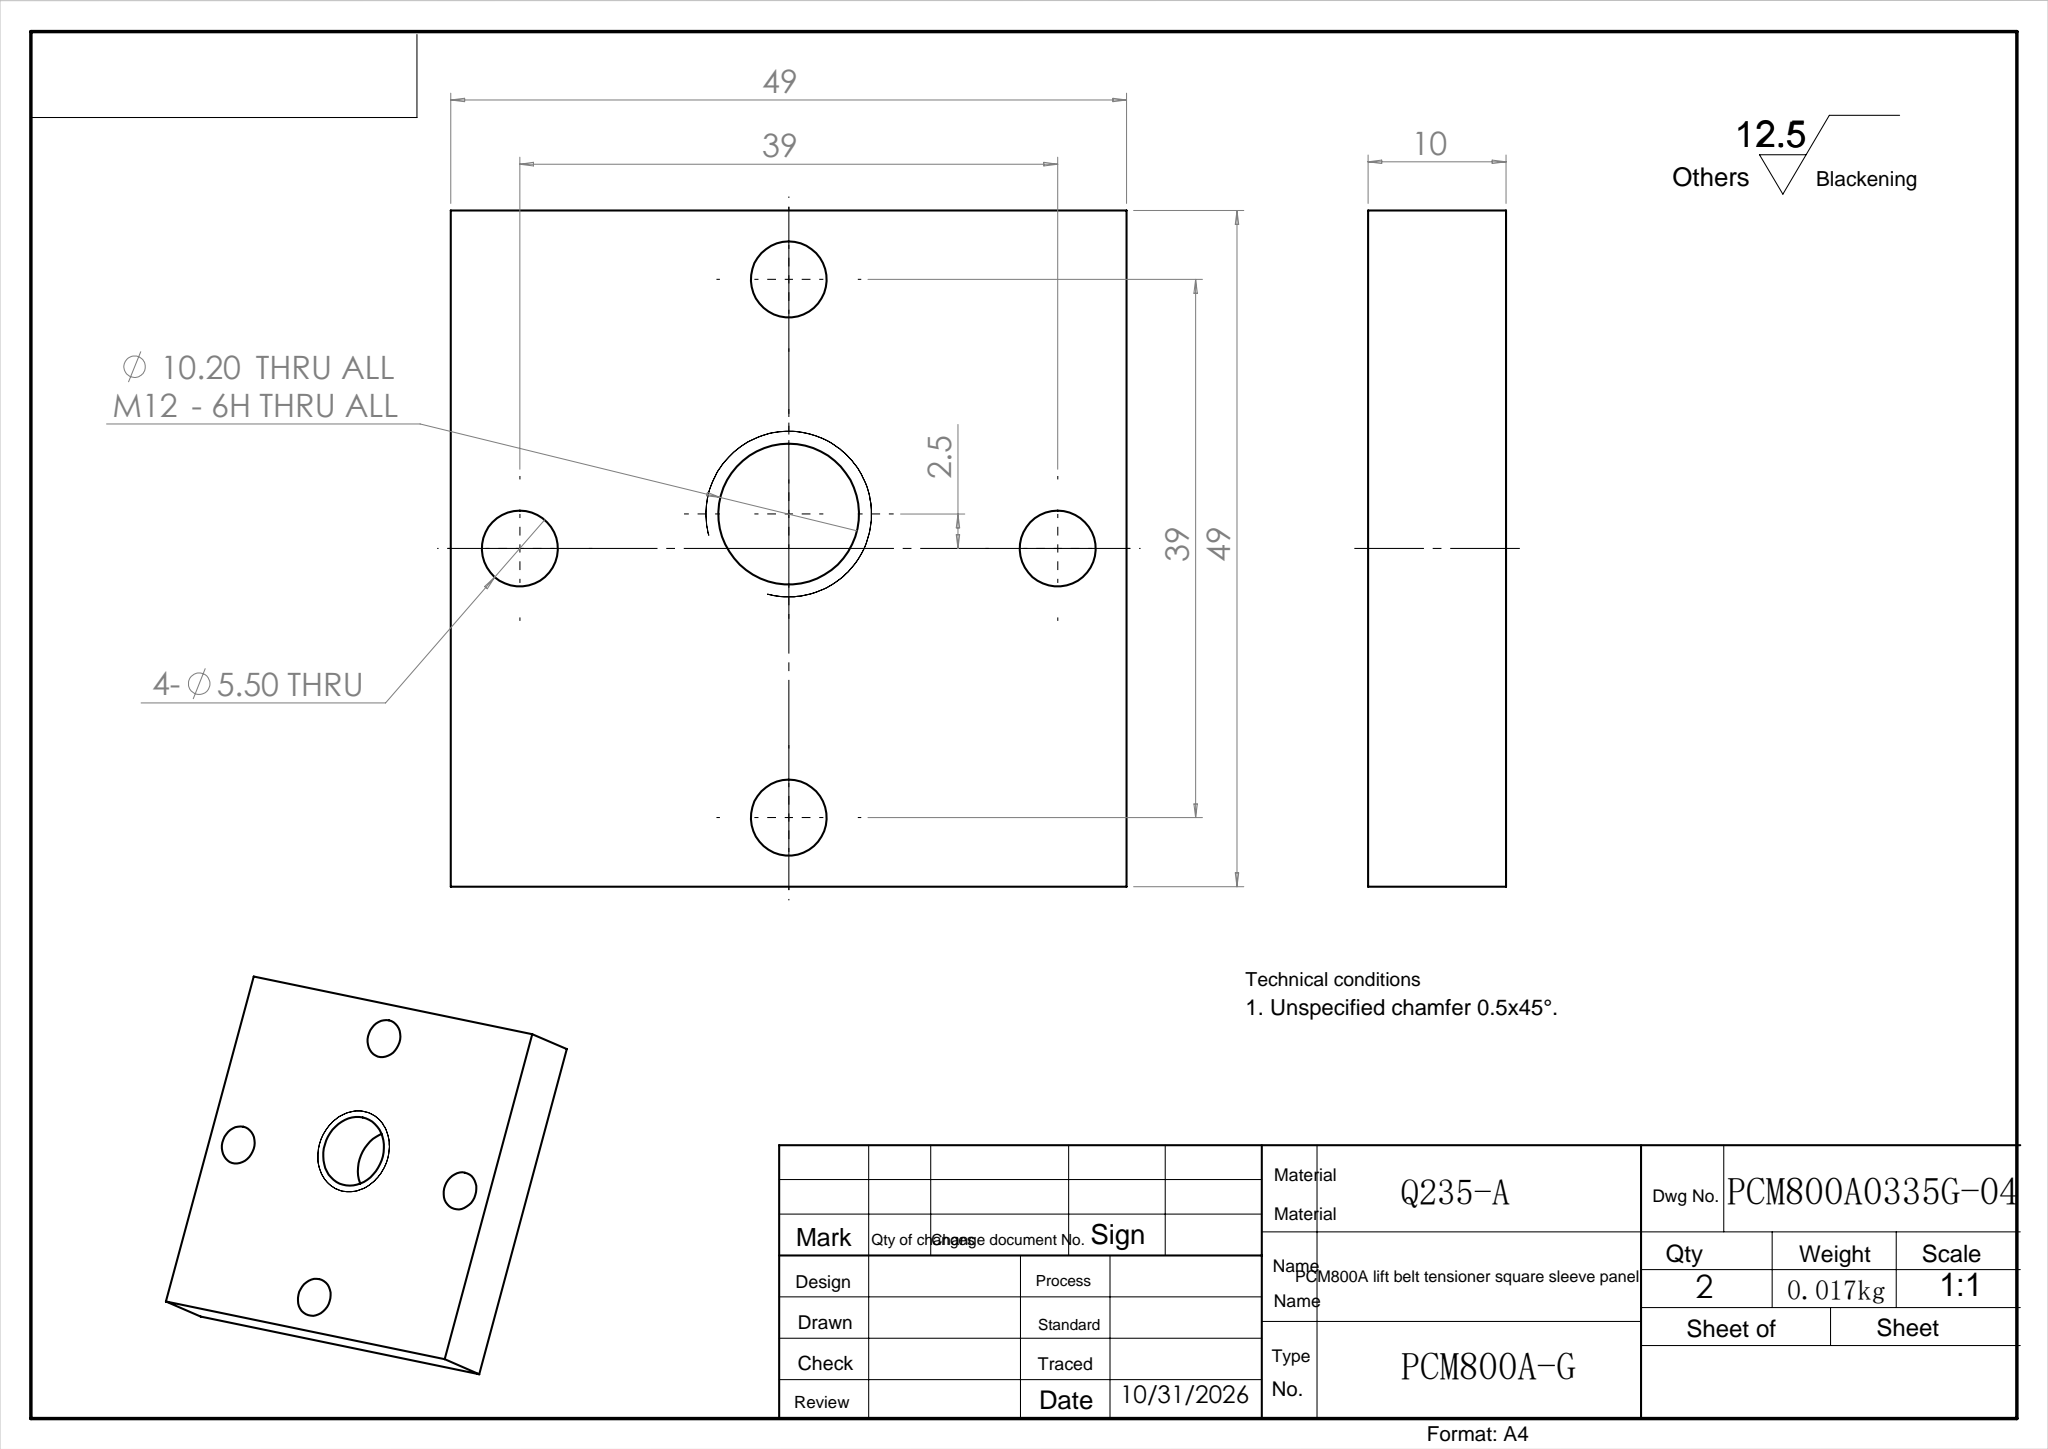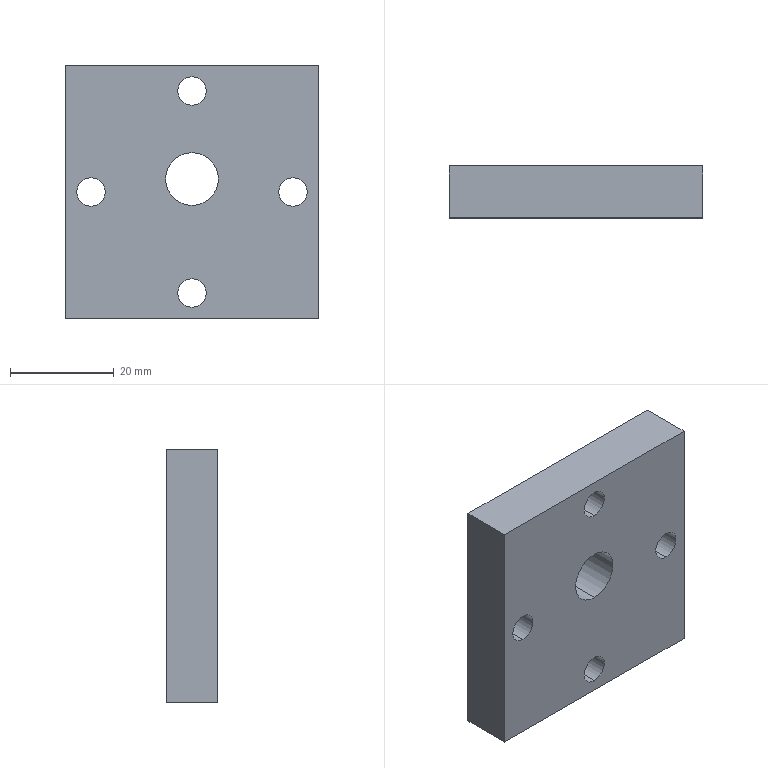Part | SolidWorks | features 3DProfileFeature 1, Cut 1, Extrusion 1, HoleWzd 1 | 1 solid | 16 faces | box 49 x 10 x 49 mm | volume 22243 mm3 | cylinder 10 | plane 6 | commonest cylinder face diameters 5.5 x8 10.2 x2
STEP:
#1=CARTESIAN_POINT('',(24.5,0.,-27.1));
#2=VERTEX_POINT('',#1);
#3=CARTESIAN_POINT('',(24.5,0.,-16.9));
#4=VERTEX_POINT('',#3);
#5=CARTESIAN_POINT('',(24.5,0.,-22.));
#6=DIRECTION('',(0.,1.,0.));
#7=DIRECTION('',(0.,0.,1.));
#8=AXIS2_PLACEMENT_3D('',#5,#6,#7);
#9=CIRCLE('',#8,5.1);
#10=EDGE_CURVE('',#2,#4,#9,.T.);
#11=ORIENTED_EDGE('',*,*,#10,.F.);
#12=CARTESIAN_POINT('',(24.5,10.,-27.1));
#13=VERTEX_POINT('',#12);
#14=CARTESIAN_POINT('',(24.5,10.,-27.1));
#15=DIRECTION('',(0.,1.,0.));
#16=VECTOR('',#15,1000.);
#17=LINE('',#14,#16);
#18=EDGE_CURVE('',#2,#13,#17,.T.);
#19=ORIENTED_EDGE('',*,*,#18,.T.);
#20=CARTESIAN_POINT('',(24.5,10.,-16.9));
#21=VERTEX_POINT('',#20);
#22=CARTESIAN_POINT('',(24.5,10.,-22.));
#23=DIRECTION('',(0.,1.,0.));
#24=DIRECTION('',(0.,0.,1.));
#25=AXIS2_PLACEMENT_3D('',#22,#23,#24);
#26=CIRCLE('',#25,5.1);
#27=EDGE_CURVE('',#13,#21,#26,.T.);
#28=ORIENTED_EDGE('',*,*,#27,.T.);
#29=CARTESIAN_POINT('',(24.5,10.,-16.9));
#30=DIRECTION('',(0.,1.,0.));
#31=VECTOR('',#30,1000.);
#32=LINE('',#29,#31);
#33=EDGE_CURVE('',#4,#21,#32,.T.);
#34=ORIENTED_EDGE('',*,*,#33,.F.);
#35=EDGE_LOOP('',(#11,#19,#28,#34));
#36=FACE_OUTER_BOUND('',#35,.T.);
#37=CARTESIAN_POINT('',(24.5,10.,-22.));
#38=DIRECTION('',(0.,1.,0.));
#39=DIRECTION('',(0.,0.,1.));
#40=AXIS2_PLACEMENT_3D('',#37,#38,#39);
#41=CYLINDRICAL_SURFACE('',#40,5.1);
#42=ADVANCED_FACE('',(#36),#41,.F.);
#43=CARTESIAN_POINT('',(5.,0.,-27.25));
#44=VERTEX_POINT('',#43);
#45=CARTESIAN_POINT('',(5.,0.,-21.75));
#46=VERTEX_POINT('',#45);
#47=CARTESIAN_POINT('',(5.,0.,-24.5));
#48=DIRECTION('',(0.,1.,0.));
#49=DIRECTION('',(0.,0.,1.));
#50=AXIS2_PLACEMENT_3D('',#47,#48,#49);
#51=CIRCLE('',#50,2.75);
#52=EDGE_CURVE('',#44,#46,#51,.T.);
#53=ORIENTED_EDGE('',*,*,#52,.F.);
#54=CARTESIAN_POINT('',(5.,10.,-27.25));
#55=VERTEX_POINT('',#54);
#56=CARTESIAN_POINT('',(5.,0.,-27.25));
#57=DIRECTION('',(0.,1.,0.));
#58=VECTOR('',#57,1000.);
#59=LINE('',#56,#58);
#60=EDGE_CURVE('',#44,#55,#59,.T.);
#61=ORIENTED_EDGE('',*,*,#60,.T.);
#62=CARTESIAN_POINT('',(5.,10.,-21.75));
#63=VERTEX_POINT('',#62);
#64=CARTESIAN_POINT('',(5.,10.,-24.5));
#65=DIRECTION('',(0.,1.,0.));
#66=DIRECTION('',(0.,0.,1.));
#67=AXIS2_PLACEMENT_3D('',#64,#65,#66);
#68=CIRCLE('',#67,2.75);
#69=EDGE_CURVE('',#55,#63,#68,.T.);
#70=ORIENTED_EDGE('',*,*,#69,.T.);
#71=CARTESIAN_POINT('',(5.,0.,-21.75));
#72=DIRECTION('',(0.,1.,0.));
#73=VECTOR('',#72,1000.);
#74=LINE('',#71,#73);
#75=EDGE_CURVE('',#46,#63,#74,.T.);
#76=ORIENTED_EDGE('',*,*,#75,.F.);
#77=EDGE_LOOP('',(#53,#61,#70,#76));
#78=FACE_OUTER_BOUND('',#77,.T.);
#79=CARTESIAN_POINT('',(5.,0.,-24.5));
#80=DIRECTION('',(0.,1.,0.));
#81=DIRECTION('',(0.,0.,1.));
#82=AXIS2_PLACEMENT_3D('',#79,#80,#81);
#83=CYLINDRICAL_SURFACE('',#82,2.75);
#84=ADVANCED_FACE('',(#78),#83,.F.);
#85=CARTESIAN_POINT('',(24.5,0.,-46.75));
#86=VERTEX_POINT('',#85);
#87=CARTESIAN_POINT('',(24.5,0.,-41.25));
#88=VERTEX_POINT('',#87);
#89=CARTESIAN_POINT('',(24.5,0.,-44.));
#90=DIRECTION('',(0.,1.,0.));
#91=DIRECTION('',(0.,0.,1.));
#92=AXIS2_PLACEMENT_3D('',#89,#90,#91);
#93=CIRCLE('',#92,2.75);
#94=EDGE_CURVE('',#86,#88,#93,.T.);
#95=ORIENTED_EDGE('',*,*,#94,.F.);
#96=CARTESIAN_POINT('',(24.5,10.,-46.75));
#97=VERTEX_POINT('',#96);
#98=CARTESIAN_POINT('',(24.5,0.,-46.75));
#99=DIRECTION('',(0.,1.,0.));
#100=VECTOR('',#99,1000.);
#101=LINE('',#98,#100);
#102=EDGE_CURVE('',#86,#97,#101,.T.);
#103=ORIENTED_EDGE('',*,*,#102,.T.);
#104=CARTESIAN_POINT('',(24.5,10.,-41.25));
#105=VERTEX_POINT('',#104);
#106=CARTESIAN_POINT('',(24.5,10.,-44.));
#107=DIRECTION('',(0.,1.,0.));
#108=DIRECTION('',(0.,0.,1.));
#109=AXIS2_PLACEMENT_3D('',#106,#107,#108);
#110=CIRCLE('',#109,2.75);
#111=EDGE_CURVE('',#97,#105,#110,.T.);
#112=ORIENTED_EDGE('',*,*,#111,.T.);
#113=CARTESIAN_POINT('',(24.5,0.,-41.25));
#114=DIRECTION('',(0.,1.,0.));
#115=VECTOR('',#114,1000.);
#116=LINE('',#113,#115);
#117=EDGE_CURVE('',#88,#105,#116,.T.);
#118=ORIENTED_EDGE('',*,*,#117,.F.);
#119=EDGE_LOOP('',(#95,#103,#112,#118));
#120=FACE_OUTER_BOUND('',#119,.T.);
#121=CARTESIAN_POINT('',(24.5,0.,-44.));
#122=DIRECTION('',(0.,1.,0.));
#123=DIRECTION('',(0.,0.,1.));
#124=AXIS2_PLACEMENT_3D('',#121,#122,#123);
#125=CYLINDRICAL_SURFACE('',#124,2.75);
#126=ADVANCED_FACE('',(#120),#125,.F.);
#127=CARTESIAN_POINT('',(44.,0.,-27.25));
#128=VERTEX_POINT('',#127);
#129=CARTESIAN_POINT('',(44.,0.,-21.75));
#130=VERTEX_POINT('',#129);
#131=CARTESIAN_POINT('',(44.,0.,-24.5));
#132=DIRECTION('',(0.,1.,0.));
#133=DIRECTION('',(0.,0.,1.));
#134=AXIS2_PLACEMENT_3D('',#131,#132,#133);
#135=CIRCLE('',#134,2.75);
#136=EDGE_CURVE('',#128,#130,#135,.T.);
#137=ORIENTED_EDGE('',*,*,#136,.F.);
#138=CARTESIAN_POINT('',(44.,10.,-27.25));
#139=VERTEX_POINT('',#138);
#140=CARTESIAN_POINT('',(44.,0.,-27.25));
#141=DIRECTION('',(0.,1.,0.));
#142=VECTOR('',#141,1000.);
#143=LINE('',#140,#142);
#144=EDGE_CURVE('',#128,#139,#143,.T.);
#145=ORIENTED_EDGE('',*,*,#144,.T.);
#146=CARTESIAN_POINT('',(44.,10.,-21.75));
#147=VERTEX_POINT('',#146);
#148=CARTESIAN_POINT('',(44.,10.,-24.5));
#149=DIRECTION('',(0.,1.,0.));
#150=DIRECTION('',(0.,0.,1.));
#151=AXIS2_PLACEMENT_3D('',#148,#149,#150);
#152=CIRCLE('',#151,2.75);
#153=EDGE_CURVE('',#139,#147,#152,.T.);
#154=ORIENTED_EDGE('',*,*,#153,.T.);
#155=CARTESIAN_POINT('',(44.,0.,-21.75));
#156=DIRECTION('',(0.,1.,0.));
#157=VECTOR('',#156,1000.);
#158=LINE('',#155,#157);
#159=EDGE_CURVE('',#130,#147,#158,.T.);
#160=ORIENTED_EDGE('',*,*,#159,.F.);
#161=EDGE_LOOP('',(#137,#145,#154,#160));
#162=FACE_OUTER_BOUND('',#161,.T.);
#163=CARTESIAN_POINT('',(44.,0.,-24.5));
#164=DIRECTION('',(0.,1.,0.));
#165=DIRECTION('',(0.,0.,1.));
#166=AXIS2_PLACEMENT_3D('',#163,#164,#165);
#167=CYLINDRICAL_SURFACE('',#166,2.75);
#168=ADVANCED_FACE('',(#162),#167,.F.);
#169=CARTESIAN_POINT('',(24.5,0.,-7.75));
#170=VERTEX_POINT('',#169);
#171=CARTESIAN_POINT('',(24.5,0.,-2.25));
#172=VERTEX_POINT('',#171);
#173=CARTESIAN_POINT('',(24.5,0.,-5.));
#174=DIRECTION('',(0.,1.,0.));
#175=DIRECTION('',(0.,0.,1.));
#176=AXIS2_PLACEMENT_3D('',#173,#174,#175);
#177=CIRCLE('',#176,2.75);
#178=EDGE_CURVE('',#170,#172,#177,.T.);
#179=ORIENTED_EDGE('',*,*,#178,.F.);
#180=CARTESIAN_POINT('',(24.5,10.,-7.75));
#181=VERTEX_POINT('',#180);
#182=CARTESIAN_POINT('',(24.5,0.,-7.75));
#183=DIRECTION('',(0.,1.,0.));
#184=VECTOR('',#183,1000.);
#185=LINE('',#182,#184);
#186=EDGE_CURVE('',#170,#181,#185,.T.);
#187=ORIENTED_EDGE('',*,*,#186,.T.);
#188=CARTESIAN_POINT('',(24.5,10.,-2.25));
#189=VERTEX_POINT('',#188);
#190=CARTESIAN_POINT('',(24.5,10.,-5.));
#191=DIRECTION('',(0.,1.,0.));
#192=DIRECTION('',(0.,0.,1.));
#193=AXIS2_PLACEMENT_3D('',#190,#191,#192);
#194=CIRCLE('',#193,2.75);
#195=EDGE_CURVE('',#181,#189,#194,.T.);
#196=ORIENTED_EDGE('',*,*,#195,.T.);
#197=CARTESIAN_POINT('',(24.5,0.,-2.25));
#198=DIRECTION('',(0.,1.,0.));
#199=VECTOR('',#198,1000.);
#200=LINE('',#197,#199);
#201=EDGE_CURVE('',#172,#189,#200,.T.);
#202=ORIENTED_EDGE('',*,*,#201,.F.);
#203=EDGE_LOOP('',(#179,#187,#196,#202));
#204=FACE_OUTER_BOUND('',#203,.T.);
#205=CARTESIAN_POINT('',(24.5,0.,-5.));
#206=DIRECTION('',(0.,1.,0.));
#207=DIRECTION('',(0.,0.,1.));
#208=AXIS2_PLACEMENT_3D('',#205,#206,#207);
#209=CYLINDRICAL_SURFACE('',#208,2.75);
#210=ADVANCED_FACE('',(#204),#209,.F.);
#211=CARTESIAN_POINT('',(0.,0.,-49.));
#212=VERTEX_POINT('',#211);
#213=CARTESIAN_POINT('',(0.,0.,0.));
#214=VERTEX_POINT('',#213);
#215=CARTESIAN_POINT('',(0.,0.,0.));
#216=DIRECTION('',(0.,0.,1.));
#217=VECTOR('',#216,1000.);
#218=LINE('',#215,#217);
#219=EDGE_CURVE('',#212,#214,#218,.T.);
#220=ORIENTED_EDGE('',*,*,#219,.F.);
#221=CARTESIAN_POINT('',(49.,0.,-49.));
#222=VERTEX_POINT('',#221);
#223=CARTESIAN_POINT('',(0.,0.,-49.));
#224=DIRECTION('',(-1.,0.,0.));
#225=VECTOR('',#224,1000.);
#226=LINE('',#223,#225);
#227=EDGE_CURVE('',#222,#212,#226,.T.);
#228=ORIENTED_EDGE('',*,*,#227,.F.);
#229=CARTESIAN_POINT('',(49.,0.,0.));
#230=VERTEX_POINT('',#229);
#231=CARTESIAN_POINT('',(49.,0.,0.));
#232=DIRECTION('',(0.,0.,-1.));
#233=VECTOR('',#232,1000.);
#234=LINE('',#231,#233);
#235=EDGE_CURVE('',#230,#222,#234,.T.);
#236=ORIENTED_EDGE('',*,*,#235,.F.);
#237=CARTESIAN_POINT('',(0.,0.,0.));
#238=DIRECTION('',(1.,0.,0.));
#239=VECTOR('',#238,1000.);
#240=LINE('',#237,#239);
#241=EDGE_CURVE('',#214,#230,#240,.T.);
#242=ORIENTED_EDGE('',*,*,#241,.F.);
#243=EDGE_LOOP('',(#220,#228,#236,#242));
#244=FACE_OUTER_BOUND('',#243,.T.);
#245=CARTESIAN_POINT('',(24.5,0.,-5.));
#246=DIRECTION('',(0.,1.,0.));
#247=DIRECTION('',(0.,0.,1.));
#248=AXIS2_PLACEMENT_3D('',#245,#246,#247);
#249=CIRCLE('',#248,2.75);
#250=EDGE_CURVE('',#172,#170,#249,.T.);
#251=ORIENTED_EDGE('',*,*,#250,.T.);
#252=ORIENTED_EDGE('',*,*,#178,.T.);
#253=EDGE_LOOP('',(#251,#252));
#254=FACE_BOUND('',#253,.T.);
#255=CARTESIAN_POINT('',(44.,0.,-24.5));
#256=DIRECTION('',(0.,1.,0.));
#257=DIRECTION('',(0.,0.,1.));
#258=AXIS2_PLACEMENT_3D('',#255,#256,#257);
#259=CIRCLE('',#258,2.75);
#260=EDGE_CURVE('',#130,#128,#259,.T.);
#261=ORIENTED_EDGE('',*,*,#260,.T.);
#262=ORIENTED_EDGE('',*,*,#136,.T.);
#263=EDGE_LOOP('',(#261,#262));
#264=FACE_BOUND('',#263,.T.);
#265=CARTESIAN_POINT('',(24.5,0.,-44.));
#266=DIRECTION('',(0.,1.,0.));
#267=DIRECTION('',(0.,0.,1.));
#268=AXIS2_PLACEMENT_3D('',#265,#266,#267);
#269=CIRCLE('',#268,2.75);
#270=EDGE_CURVE('',#88,#86,#269,.T.);
#271=ORIENTED_EDGE('',*,*,#270,.T.);
#272=ORIENTED_EDGE('',*,*,#94,.T.);
#273=EDGE_LOOP('',(#271,#272));
#274=FACE_BOUND('',#273,.T.);
#275=CARTESIAN_POINT('',(5.,0.,-24.5));
#276=DIRECTION('',(0.,1.,0.));
#277=DIRECTION('',(0.,0.,1.));
#278=AXIS2_PLACEMENT_3D('',#275,#276,#277);
#279=CIRCLE('',#278,2.75);
#280=EDGE_CURVE('',#46,#44,#279,.T.);
#281=ORIENTED_EDGE('',*,*,#280,.T.);
#282=ORIENTED_EDGE('',*,*,#52,.T.);
#283=EDGE_LOOP('',(#281,#282));
#284=FACE_BOUND('',#283,.T.);
#285=CARTESIAN_POINT('',(24.5,0.,-22.));
#286=DIRECTION('',(0.,1.,0.));
#287=DIRECTION('',(0.,0.,1.));
#288=AXIS2_PLACEMENT_3D('',#285,#286,#287);
#289=CIRCLE('',#288,5.1);
#290=EDGE_CURVE('',#4,#2,#289,.T.);
#291=ORIENTED_EDGE('',*,*,#290,.T.);
#292=ORIENTED_EDGE('',*,*,#10,.T.);
#293=EDGE_LOOP('',(#291,#292));
#294=FACE_BOUND('',#293,.T.);
#295=CARTESIAN_POINT('',(0.,0.,-49.));
#296=DIRECTION('',(0.,-1.,0.));
#297=DIRECTION('',(0.,0.,-1.));
#298=AXIS2_PLACEMENT_3D('',#295,#296,#297);
#299=PLANE('',#298);
#300=ADVANCED_FACE('',(#244,#254,#264,#274,#284,#294),#299,.T.);
#301=ORIENTED_EDGE('',*,*,#219,.T.);
#302=CARTESIAN_POINT('',(0.,10.,0.));
#303=VERTEX_POINT('',#302);
#304=CARTESIAN_POINT('',(0.,10.,0.));
#305=DIRECTION('',(0.,-1.,0.));
#306=VECTOR('',#305,1000.);
#307=LINE('',#304,#306);
#308=EDGE_CURVE('',#303,#214,#307,.T.);
#309=ORIENTED_EDGE('',*,*,#308,.F.);
#310=CARTESIAN_POINT('',(0.,10.,-49.));
#311=VERTEX_POINT('',#310);
#312=CARTESIAN_POINT('',(0.,10.,0.));
#313=DIRECTION('',(0.,0.,1.));
#314=VECTOR('',#313,1000.);
#315=LINE('',#312,#314);
#316=EDGE_CURVE('',#311,#303,#315,.T.);
#317=ORIENTED_EDGE('',*,*,#316,.F.);
#318=CARTESIAN_POINT('',(0.,10.,-49.));
#319=DIRECTION('',(0.,-1.,0.));
#320=VECTOR('',#319,1000.);
#321=LINE('',#318,#320);
#322=EDGE_CURVE('',#311,#212,#321,.T.);
#323=ORIENTED_EDGE('',*,*,#322,.T.);
#324=EDGE_LOOP('',(#301,#309,#317,#323));
#325=FACE_OUTER_BOUND('',#324,.T.);
#326=CARTESIAN_POINT('',(0.,10.,0.));
#327=DIRECTION('',(1.,0.,0.));
#328=DIRECTION('',(0.,0.,-1.));
#329=AXIS2_PLACEMENT_3D('',#326,#327,#328);
#330=PLANE('',#329);
#331=ADVANCED_FACE('',(#325),#330,.F.);
#332=ORIENTED_EDGE('',*,*,#241,.T.);
#333=CARTESIAN_POINT('',(49.,10.,0.));
#334=VERTEX_POINT('',#333);
#335=CARTESIAN_POINT('',(49.,10.,0.));
#336=DIRECTION('',(0.,-1.,0.));
#337=VECTOR('',#336,1000.);
#338=LINE('',#335,#337);
#339=EDGE_CURVE('',#334,#230,#338,.T.);
#340=ORIENTED_EDGE('',*,*,#339,.F.);
#341=CARTESIAN_POINT('',(0.,10.,0.));
#342=DIRECTION('',(1.,0.,0.));
#343=VECTOR('',#342,1000.);
#344=LINE('',#341,#343);
#345=EDGE_CURVE('',#303,#334,#344,.T.);
#346=ORIENTED_EDGE('',*,*,#345,.F.);
#347=ORIENTED_EDGE('',*,*,#308,.T.);
#348=EDGE_LOOP('',(#332,#340,#346,#347));
#349=FACE_OUTER_BOUND('',#348,.T.);
#350=CARTESIAN_POINT('',(0.,10.,0.));
#351=DIRECTION('',(0.,0.,-1.));
#352=DIRECTION('',(-1.,0.,0.));
#353=AXIS2_PLACEMENT_3D('',#350,#351,#352);
#354=PLANE('',#353);
#355=ADVANCED_FACE('',(#349),#354,.F.);
#356=ORIENTED_EDGE('',*,*,#235,.T.);
#357=CARTESIAN_POINT('',(49.,10.,-49.));
#358=VERTEX_POINT('',#357);
#359=CARTESIAN_POINT('',(49.,10.,-49.));
#360=DIRECTION('',(0.,-1.,0.));
#361=VECTOR('',#360,1000.);
#362=LINE('',#359,#361);
#363=EDGE_CURVE('',#358,#222,#362,.T.);
#364=ORIENTED_EDGE('',*,*,#363,.F.);
#365=CARTESIAN_POINT('',(49.,10.,0.));
#366=DIRECTION('',(0.,0.,-1.));
#367=VECTOR('',#366,1000.);
#368=LINE('',#365,#367);
#369=EDGE_CURVE('',#334,#358,#368,.T.);
#370=ORIENTED_EDGE('',*,*,#369,.F.);
#371=ORIENTED_EDGE('',*,*,#339,.T.);
#372=EDGE_LOOP('',(#356,#364,#370,#371));
#373=FACE_OUTER_BOUND('',#372,.T.);
#374=CARTESIAN_POINT('',(49.,10.,0.));
#375=DIRECTION('',(-1.,0.,0.));
#376=DIRECTION('',(0.,0.,1.));
#377=AXIS2_PLACEMENT_3D('',#374,#375,#376);
#378=PLANE('',#377);
#379=ADVANCED_FACE('',(#373),#378,.F.);
#380=ORIENTED_EDGE('',*,*,#227,.T.);
#381=ORIENTED_EDGE('',*,*,#322,.F.);
#382=CARTESIAN_POINT('',(0.,10.,-49.));
#383=DIRECTION('',(-1.,0.,0.));
#384=VECTOR('',#383,1000.);
#385=LINE('',#382,#384);
#386=EDGE_CURVE('',#358,#311,#385,.T.);
#387=ORIENTED_EDGE('',*,*,#386,.F.);
#388=ORIENTED_EDGE('',*,*,#363,.T.);
#389=EDGE_LOOP('',(#380,#381,#387,#388));
#390=FACE_OUTER_BOUND('',#389,.T.);
#391=CARTESIAN_POINT('',(0.,10.,-49.));
#392=DIRECTION('',(0.,0.,1.));
#393=DIRECTION('',(1.,0.,0.));
#394=AXIS2_PLACEMENT_3D('',#391,#392,#393);
#395=PLANE('',#394);
#396=ADVANCED_FACE('',(#390),#395,.F.);
#397=CARTESIAN_POINT('',(24.5,10.,-22.));
#398=DIRECTION('',(0.,1.,0.));
#399=DIRECTION('',(0.,0.,1.));
#400=AXIS2_PLACEMENT_3D('',#397,#398,#399);
#401=CIRCLE('',#400,5.1);
#402=EDGE_CURVE('',#21,#13,#401,.T.);
#403=ORIENTED_EDGE('',*,*,#402,.F.);
#404=ORIENTED_EDGE('',*,*,#27,.F.);
#405=EDGE_LOOP('',(#403,#404));
#406=FACE_BOUND('',#405,.T.);
#407=CARTESIAN_POINT('',(5.,10.,-24.5));
#408=DIRECTION('',(0.,1.,0.));
#409=DIRECTION('',(0.,0.,1.));
#410=AXIS2_PLACEMENT_3D('',#407,#408,#409);
#411=CIRCLE('',#410,2.75);
#412=EDGE_CURVE('',#63,#55,#411,.T.);
#413=ORIENTED_EDGE('',*,*,#412,.F.);
#414=ORIENTED_EDGE('',*,*,#69,.F.);
#415=EDGE_LOOP('',(#413,#414));
#416=FACE_BOUND('',#415,.T.);
#417=CARTESIAN_POINT('',(24.5,10.,-44.));
#418=DIRECTION('',(0.,1.,0.));
#419=DIRECTION('',(0.,0.,1.));
#420=AXIS2_PLACEMENT_3D('',#417,#418,#419);
#421=CIRCLE('',#420,2.75);
#422=EDGE_CURVE('',#105,#97,#421,.T.);
#423=ORIENTED_EDGE('',*,*,#422,.F.);
#424=ORIENTED_EDGE('',*,*,#111,.F.);
#425=EDGE_LOOP('',(#423,#424));
#426=FACE_BOUND('',#425,.T.);
#427=CARTESIAN_POINT('',(44.,10.,-24.5));
#428=DIRECTION('',(0.,1.,0.));
#429=DIRECTION('',(0.,0.,1.));
#430=AXIS2_PLACEMENT_3D('',#427,#428,#429);
#431=CIRCLE('',#430,2.75);
#432=EDGE_CURVE('',#147,#139,#431,.T.);
#433=ORIENTED_EDGE('',*,*,#432,.F.);
#434=ORIENTED_EDGE('',*,*,#153,.F.);
#435=EDGE_LOOP('',(#433,#434));
#436=FACE_BOUND('',#435,.T.);
#437=CARTESIAN_POINT('',(24.5,10.,-5.));
#438=DIRECTION('',(0.,1.,0.));
#439=DIRECTION('',(0.,0.,1.));
#440=AXIS2_PLACEMENT_3D('',#437,#438,#439);
#441=CIRCLE('',#440,2.75);
#442=EDGE_CURVE('',#189,#181,#441,.T.);
#443=ORIENTED_EDGE('',*,*,#442,.F.);
#444=ORIENTED_EDGE('',*,*,#195,.F.);
#445=EDGE_LOOP('',(#443,#444));
#446=FACE_BOUND('',#445,.T.);
#447=ORIENTED_EDGE('',*,*,#316,.T.);
#448=ORIENTED_EDGE('',*,*,#345,.T.);
#449=ORIENTED_EDGE('',*,*,#369,.T.);
#450=ORIENTED_EDGE('',*,*,#386,.T.);
#451=EDGE_LOOP('',(#447,#448,#449,#450));
#452=FACE_OUTER_BOUND('',#451,.T.);
#453=CARTESIAN_POINT('',(0.,10.,-49.));
#454=DIRECTION('',(0.,-1.,0.));
#455=DIRECTION('',(0.,0.,-1.));
#456=AXIS2_PLACEMENT_3D('',#453,#454,#455);
#457=PLANE('',#456);
#458=ADVANCED_FACE('',(#406,#416,#426,#436,#446,#452),#457,.F.);
#459=ORIENTED_EDGE('',*,*,#186,.F.);
#460=ORIENTED_EDGE('',*,*,#250,.F.);
#461=ORIENTED_EDGE('',*,*,#201,.T.);
#462=ORIENTED_EDGE('',*,*,#442,.T.);
#463=EDGE_LOOP('',(#459,#460,#461,#462));
#464=FACE_OUTER_BOUND('',#463,.T.);
#465=CARTESIAN_POINT('',(24.5,0.,-5.));
#466=DIRECTION('',(0.,1.,0.));
#467=DIRECTION('',(0.,0.,1.));
#468=AXIS2_PLACEMENT_3D('',#465,#466,#467);
#469=CYLINDRICAL_SURFACE('',#468,2.75);
#470=ADVANCED_FACE('',(#464),#469,.F.);
#471=ORIENTED_EDGE('',*,*,#144,.F.);
#472=ORIENTED_EDGE('',*,*,#260,.F.);
#473=ORIENTED_EDGE('',*,*,#159,.T.);
#474=ORIENTED_EDGE('',*,*,#432,.T.);
#475=EDGE_LOOP('',(#471,#472,#473,#474));
#476=FACE_OUTER_BOUND('',#475,.T.);
#477=CARTESIAN_POINT('',(44.,0.,-24.5));
#478=DIRECTION('',(0.,1.,0.));
#479=DIRECTION('',(0.,0.,1.));
#480=AXIS2_PLACEMENT_3D('',#477,#478,#479);
#481=CYLINDRICAL_SURFACE('',#480,2.75);
#482=ADVANCED_FACE('',(#476),#481,.F.);
#483=ORIENTED_EDGE('',*,*,#102,.F.);
#484=ORIENTED_EDGE('',*,*,#270,.F.);
#485=ORIENTED_EDGE('',*,*,#117,.T.);
#486=ORIENTED_EDGE('',*,*,#422,.T.);
#487=EDGE_LOOP('',(#483,#484,#485,#486));
#488=FACE_OUTER_BOUND('',#487,.T.);
#489=CARTESIAN_POINT('',(24.5,0.,-44.));
#490=DIRECTION('',(0.,1.,0.));
#491=DIRECTION('',(0.,0.,1.));
#492=AXIS2_PLACEMENT_3D('',#489,#490,#491);
#493=CYLINDRICAL_SURFACE('',#492,2.75);
#494=ADVANCED_FACE('',(#488),#493,.F.);
#495=ORIENTED_EDGE('',*,*,#60,.F.);
#496=ORIENTED_EDGE('',*,*,#280,.F.);
#497=ORIENTED_EDGE('',*,*,#75,.T.);
#498=ORIENTED_EDGE('',*,*,#412,.T.);
#499=EDGE_LOOP('',(#495,#496,#497,#498));
#500=FACE_OUTER_BOUND('',#499,.T.);
#501=CARTESIAN_POINT('',(5.,0.,-24.5));
#502=DIRECTION('',(0.,1.,0.));
#503=DIRECTION('',(0.,0.,1.));
#504=AXIS2_PLACEMENT_3D('',#501,#502,#503);
#505=CYLINDRICAL_SURFACE('',#504,2.75);
#506=ADVANCED_FACE('',(#500),#505,.F.);
#507=ORIENTED_EDGE('',*,*,#18,.F.);
#508=ORIENTED_EDGE('',*,*,#290,.F.);
#509=ORIENTED_EDGE('',*,*,#33,.T.);
#510=ORIENTED_EDGE('',*,*,#402,.T.);
#511=EDGE_LOOP('',(#507,#508,#509,#510));
#512=FACE_OUTER_BOUND('',#511,.T.);
#513=CARTESIAN_POINT('',(24.5,10.,-22.));
#514=DIRECTION('',(0.,1.,0.));
#515=DIRECTION('',(0.,0.,1.));
#516=AXIS2_PLACEMENT_3D('',#513,#514,#515);
#517=CYLINDRICAL_SURFACE('',#516,5.1);
#518=ADVANCED_FACE('',(#512),#517,.F.);
#519=CLOSED_SHELL('',(#42,#84,#126,#168,#210,#300,#331,#355,#379,#396,#458,#470,#482,#494,#506,#518));
#520=MANIFOLD_SOLID_BREP('',#519);
#521=CARTESIAN_POINT('',(0.,0.,0.));
#522=DIRECTION('',(0.,0.,1.));
#523=DIRECTION('',(1.,0.,0.));
#524=AXIS2_PLACEMENT_3D('',#521,#522,#523);
#525=(LENGTH_UNIT()NAMED_UNIT(*)SI_UNIT(.MILLI.,.METRE.));
#526=UNCERTAINTY_MEASURE_WITH_UNIT(LENGTH_MEASURE(0.00001),#525,'','');
#527=(NAMED_UNIT(*)PLANE_ANGLE_UNIT()SI_UNIT($,.RADIAN.));
#528=(NAMED_UNIT(*)SI_UNIT($,.STERADIAN.)SOLID_ANGLE_UNIT());
#529=(GEOMETRIC_REPRESENTATION_CONTEXT(3)GLOBAL_UNCERTAINTY_ASSIGNED_CONTEXT((#526))GLOBAL_UNIT_ASSIGNED_CONTEXT((#525,#527,#528))REPRESENTATION_CONTEXT('',''));
#530=ADVANCED_BREP_SHAPE_REPRESENTATION('',(#520,#524),#529);